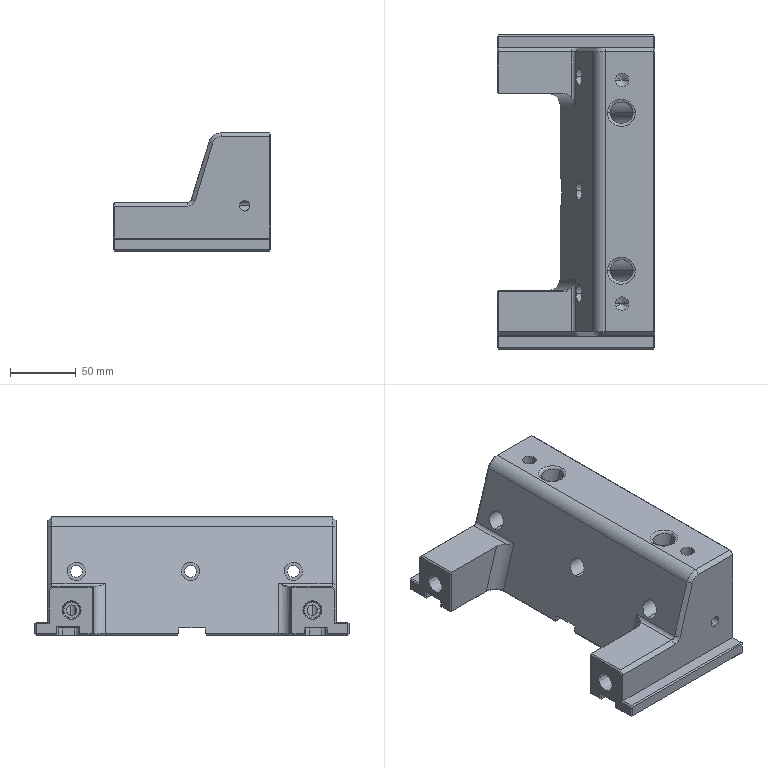Part | Creo | 1 solid | 249 faces | box 120 x 239 x 90 mm | volume 1169735 mm3 | plane 132 | cylinder 73 | cone 28 | spline 12 | torus 4 | commonest cylinder face diameters 8 x18 6 x10 1.5 x8 9 x6 14 x6 1 x4